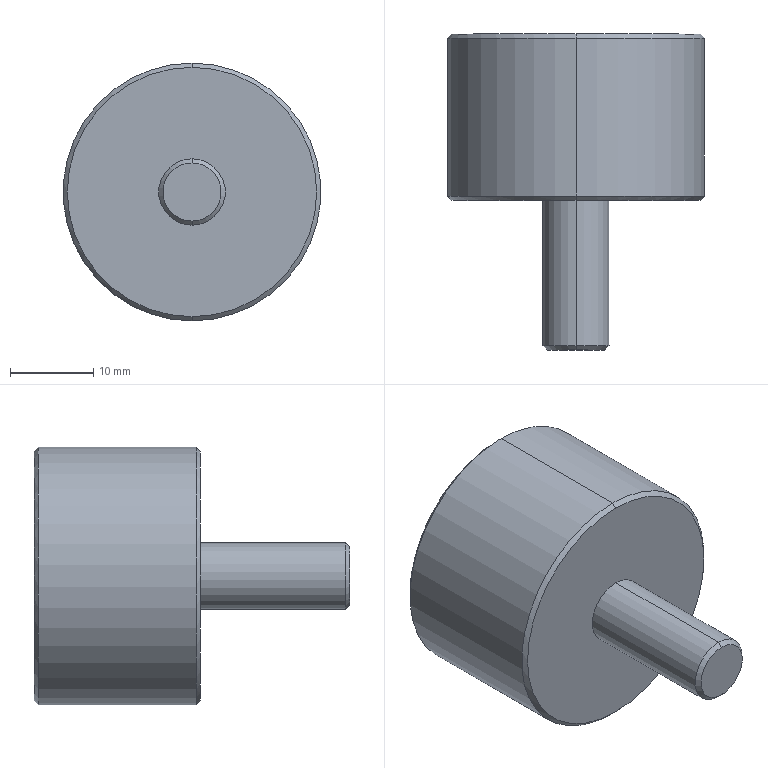Part | STEP file | OP10-123_seal rod | 1 solid | 23 faces | box 31 x 38 x 31 mm | volume 15633 mm3 | cylinder 10 | cone 8 | plane 5 | commonest cylinder face diameters 3.3 x2 6 x2 8 x2 11 x2 31 x2
STEP:
#1=CARTESIAN_POINT('',(0.,0.,0.));
#2=DIRECTION('',(0.,0.,1.));
#3=DIRECTION('',(1.,0.,0.));
#4=AXIS2_PLACEMENT_3D('',#1,#2,#3);
#5=CARTESIAN_POINT('',(0.,0.,-3.5));
#6=VERTEX_POINT('',#5);
#7=CARTESIAN_POINT('',(0.,0.,3.5));
#8=VERTEX_POINT('',#7);
#9=CARTESIAN_POINT('',(0.,0.,0.));
#10=DIRECTION('',(0.,-1.,0.));
#11=DIRECTION('',(0.,0.,1.));
#12=AXIS2_PLACEMENT_3D('',#9,#10,#11);
#13=CIRCLE('',#12,3.5);
#14=CARTESIAN_POINT('',(0.,0.5,0.));
#15=DIRECTION('',(0.,1.,0.));
#16=DIRECTION('',(0.,0.,1.));
#17=AXIS2_PLACEMENT_3D('',#14,#15,#16);
#18=CONICAL_SURFACE('',#17,4.,0.7854);
#19=CARTESIAN_POINT('',(6.283,-0.5));
#20=DIRECTION('',(-1.,0.));
#21=VECTOR('',#20,1.);
#22=LINE('',#19,#21);
#23=(GEOMETRIC_REPRESENTATION_CONTEXT(2)PARAMETRIC_REPRESENTATION_CONTEXT()REPRESENTATION_CONTEXT('',''));
#24=DEFINITIONAL_REPRESENTATION('',(#22),#23);
#25=PCURVE('',#18,#24);
#26=CARTESIAN_POINT('',(0.,0.,0.));
#27=DIRECTION('',(0.,1.,0.));
#28=DIRECTION('',(0.,0.,1.));
#29=AXIS2_PLACEMENT_3D('',#26,#27,#28);
#30=PLANE('',#29);
#31=CARTESIAN_POINT('',(3.5,0.));
#32=CARTESIAN_POINT('',(3.5,-6.062));
#33=CARTESIAN_POINT('',(-1.75,-3.031));
#34=CARTESIAN_POINT('',(-7.,0.));
#35=CARTESIAN_POINT('',(-1.75,3.031));
#36=CARTESIAN_POINT('',(3.5,6.062));
#37=CARTESIAN_POINT('',(3.5,0.));
#38=(BOUNDED_CURVE()B_SPLINE_CURVE(2,(#31,#32,#33,#34,#35,#36,#37),.UNSPECIFIED.,.T.,.F.)B_SPLINE_CURVE_WITH_KNOTS((1,2,2,2,2,1),(-2.094,0.,2.094,4.189,6.283,8.378),.UNSPECIFIED.)CURVE()GEOMETRIC_REPRESENTATION_ITEM()RATIONAL_B_SPLINE_CURVE((1.,0.5,1.,0.5,1.,0.5,1.))REPRESENTATION_ITEM(''));
#39=(GEOMETRIC_REPRESENTATION_CONTEXT(2)PARAMETRIC_REPRESENTATION_CONTEXT()REPRESENTATION_CONTEXT('',''));
#40=DEFINITIONAL_REPRESENTATION('',(#38),#39);
#41=PCURVE('',#30,#40);
#42=SURFACE_CURVE('',#13,(#25,#41),.PCURVE_S1.);
#43=EDGE_CURVE('',#6,#8,#42,.T.);
#44=ORIENTED_EDGE('',*,*,#43,.F.);
#45=CARTESIAN_POINT('',(0.,0.5,-4.));
#46=VERTEX_POINT('',#45);
#47=CARTESIAN_POINT('',(0.,0.5,-4.));
#48=DIRECTION('',(0.,0.7071,-0.7071));
#49=VECTOR('',#48,1.);
#50=LINE('',#47,#49);
#51=CARTESIAN_POINT('',(3.142,0.));
#52=DIRECTION('',(0.,1.));
#53=VECTOR('',#52,1.);
#54=LINE('',#51,#53);
#55=(GEOMETRIC_REPRESENTATION_CONTEXT(2)PARAMETRIC_REPRESENTATION_CONTEXT()REPRESENTATION_CONTEXT('',''));
#56=DEFINITIONAL_REPRESENTATION('',(#54),#55);
#57=PCURVE('',#18,#56);
#58=CARTESIAN_POINT('',(0.,0.5,0.));
#59=DIRECTION('',(0.,1.,0.));
#60=DIRECTION('',(0.,0.,1.));
#61=AXIS2_PLACEMENT_3D('',#58,#59,#60);
#62=CONICAL_SURFACE('',#61,4.,0.7854);
#63=CARTESIAN_POINT('',(3.142,0.));
#64=DIRECTION('',(0.,1.));
#65=VECTOR('',#64,1.);
#66=LINE('',#63,#65);
#67=(GEOMETRIC_REPRESENTATION_CONTEXT(2)PARAMETRIC_REPRESENTATION_CONTEXT()REPRESENTATION_CONTEXT('',''));
#68=DEFINITIONAL_REPRESENTATION('',(#66),#67);
#69=PCURVE('',#62,#68);
#70=SURFACE_CURVE('',#50,(#57,#69),.PCURVE_S1.);
#71=EDGE_CURVE('',#6,#46,#70,.T.);
#72=ORIENTED_EDGE('',*,*,#71,.T.);
#73=CARTESIAN_POINT('',(0.,0.5,4.));
#74=VERTEX_POINT('',#73);
#75=CARTESIAN_POINT('',(0.,0.5,0.));
#76=DIRECTION('',(0.,1.,0.));
#77=DIRECTION('',(0.,0.,1.));
#78=AXIS2_PLACEMENT_3D('',#75,#76,#77);
#79=CIRCLE('',#78,4.);
#80=CARTESIAN_POINT('',(0.,0.));
#81=DIRECTION('',(1.,0.));
#82=VECTOR('',#81,1.);
#83=LINE('',#80,#82);
#84=(GEOMETRIC_REPRESENTATION_CONTEXT(2)PARAMETRIC_REPRESENTATION_CONTEXT()REPRESENTATION_CONTEXT('',''));
#85=DEFINITIONAL_REPRESENTATION('',(#83),#84);
#86=PCURVE('',#18,#85);
#87=CARTESIAN_POINT('',(0.,18.,0.));
#88=DIRECTION('',(0.,-1.,0.));
#89=DIRECTION('',(0.,0.,-1.));
#90=AXIS2_PLACEMENT_3D('',#87,#88,#89);
#91=CYLINDRICAL_SURFACE('',#90,4.);
#92=CARTESIAN_POINT('',(3.142,17.5));
#93=DIRECTION('',(-1.,0.));
#94=VECTOR('',#93,1.);
#95=LINE('',#92,#94);
#96=(GEOMETRIC_REPRESENTATION_CONTEXT(2)PARAMETRIC_REPRESENTATION_CONTEXT()REPRESENTATION_CONTEXT('',''));
#97=DEFINITIONAL_REPRESENTATION('',(#95),#96);
#98=PCURVE('',#91,#97);
#99=SURFACE_CURVE('',#79,(#86,#98),.PCURVE_S1.);
#100=EDGE_CURVE('',#74,#46,#99,.T.);
#101=ORIENTED_EDGE('',*,*,#100,.F.);
#102=CARTESIAN_POINT('',(0.,0.5,4.));
#103=DIRECTION('',(0.,0.7071,0.7071));
#104=VECTOR('',#103,1.);
#105=LINE('',#102,#104);
#106=CARTESIAN_POINT('',(0.,0.));
#107=DIRECTION('',(0.,1.));
#108=VECTOR('',#107,1.);
#109=LINE('',#106,#108);
#110=(GEOMETRIC_REPRESENTATION_CONTEXT(2)PARAMETRIC_REPRESENTATION_CONTEXT()REPRESENTATION_CONTEXT('',''));
#111=DEFINITIONAL_REPRESENTATION('',(#109),#110);
#112=PCURVE('',#18,#111);
#113=CARTESIAN_POINT('',(6.283,0.));
#114=DIRECTION('',(0.,1.));
#115=VECTOR('',#114,1.);
#116=LINE('',#113,#115);
#117=(GEOMETRIC_REPRESENTATION_CONTEXT(2)PARAMETRIC_REPRESENTATION_CONTEXT()REPRESENTATION_CONTEXT('',''));
#118=DEFINITIONAL_REPRESENTATION('',(#116),#117);
#119=PCURVE('',#62,#118);
#120=SURFACE_CURVE('',#105,(#112,#119),.PCURVE_S1.);
#121=EDGE_CURVE('',#8,#74,#120,.T.);
#122=ORIENTED_EDGE('',*,*,#121,.F.);
#123=EDGE_LOOP('',(#44,#72,#101,#122));
#124=FACE_BOUND('',#123,.T.);
#125=ADVANCED_FACE('',(#124),#18,.T.);
#126=CARTESIAN_POINT('',(0.,38.,15.));
#127=VERTEX_POINT('',#126);
#128=CARTESIAN_POINT('',(0.,38.,-15.));
#129=VERTEX_POINT('',#128);
#130=CARTESIAN_POINT('',(0.,38.,0.));
#131=DIRECTION('',(0.,1.,0.));
#132=DIRECTION('',(0.,0.,1.));
#133=AXIS2_PLACEMENT_3D('',#130,#131,#132);
#134=CIRCLE('',#133,15.);
#135=CARTESIAN_POINT('',(0.,38.,0.));
#136=DIRECTION('',(0.,-1.,0.));
#137=DIRECTION('',(0.,0.,-1.));
#138=AXIS2_PLACEMENT_3D('',#135,#136,#137);
#139=CONICAL_SURFACE('',#138,15.,0.7854);
#140=CARTESIAN_POINT('',(3.142,0.));
#141=DIRECTION('',(-1.,0.));
#142=VECTOR('',#141,1.);
#143=LINE('',#140,#142);
#144=(GEOMETRIC_REPRESENTATION_CONTEXT(2)PARAMETRIC_REPRESENTATION_CONTEXT()REPRESENTATION_CONTEXT('',''));
#145=DEFINITIONAL_REPRESENTATION('',(#143),#144);
#146=PCURVE('',#139,#145);
#147=CARTESIAN_POINT('',(0.,38.,0.));
#148=DIRECTION('',(0.,1.,0.));
#149=DIRECTION('',(0.,0.,1.));
#150=AXIS2_PLACEMENT_3D('',#147,#148,#149);
#151=PLANE('',#150);
#152=CARTESIAN_POINT('',(0.,0.));
#153=DIRECTION('',(1.,0.));
#154=AXIS2_PLACEMENT_2D('',#152,#153);
#155=CIRCLE('',#154,15.);
#156=(GEOMETRIC_REPRESENTATION_CONTEXT(2)PARAMETRIC_REPRESENTATION_CONTEXT()REPRESENTATION_CONTEXT('',''));
#157=DEFINITIONAL_REPRESENTATION('',(#155),#156);
#158=PCURVE('',#151,#157);
#159=SURFACE_CURVE('',#134,(#146,#158),.PCURVE_S1.);
#160=EDGE_CURVE('',#127,#129,#159,.T.);
#161=ORIENTED_EDGE('',*,*,#160,.F.);
#162=CARTESIAN_POINT('',(0.,37.5,15.5));
#163=VERTEX_POINT('',#162);
#164=CARTESIAN_POINT('',(0.,38.,15.));
#165=DIRECTION('',(0.,-0.7071,0.7071));
#166=VECTOR('',#165,1.);
#167=LINE('',#164,#166);
#168=CARTESIAN_POINT('',(3.142,0.));
#169=DIRECTION('',(0.,1.));
#170=VECTOR('',#169,1.);
#171=LINE('',#168,#170);
#172=(GEOMETRIC_REPRESENTATION_CONTEXT(2)PARAMETRIC_REPRESENTATION_CONTEXT()REPRESENTATION_CONTEXT('',''));
#173=DEFINITIONAL_REPRESENTATION('',(#171),#172);
#174=PCURVE('',#139,#173);
#175=CARTESIAN_POINT('',(0.,38.,0.));
#176=DIRECTION('',(0.,-1.,0.));
#177=DIRECTION('',(0.,0.,-1.));
#178=AXIS2_PLACEMENT_3D('',#175,#176,#177);
#179=CONICAL_SURFACE('',#178,15.,0.7854);
#180=CARTESIAN_POINT('',(3.142,0.));
#181=DIRECTION('',(0.,1.));
#182=VECTOR('',#181,1.);
#183=LINE('',#180,#182);
#184=(GEOMETRIC_REPRESENTATION_CONTEXT(2)PARAMETRIC_REPRESENTATION_CONTEXT()REPRESENTATION_CONTEXT('',''));
#185=DEFINITIONAL_REPRESENTATION('',(#183),#184);
#186=PCURVE('',#179,#185);
#187=SURFACE_CURVE('',#167,(#174,#186),.PCURVE_S1.);
#188=EDGE_CURVE('',#127,#163,#187,.T.);
#189=ORIENTED_EDGE('',*,*,#188,.T.);
#190=CARTESIAN_POINT('',(0.,37.5,-15.5));
#191=VERTEX_POINT('',#190);
#192=CARTESIAN_POINT('',(0.,37.5,0.));
#193=DIRECTION('',(0.,-1.,0.));
#194=DIRECTION('',(0.,0.,1.));
#195=AXIS2_PLACEMENT_3D('',#192,#193,#194);
#196=CIRCLE('',#195,15.5);
#197=CARTESIAN_POINT('',(-3.142,0.5));
#198=DIRECTION('',(1.,0.));
#199=VECTOR('',#198,1.);
#200=LINE('',#197,#199);
#201=(GEOMETRIC_REPRESENTATION_CONTEXT(2)PARAMETRIC_REPRESENTATION_CONTEXT()REPRESENTATION_CONTEXT('',''));
#202=DEFINITIONAL_REPRESENTATION('',(#200),#201);
#203=PCURVE('',#139,#202);
#204=CARTESIAN_POINT('',(0.,38.,0.));
#205=DIRECTION('',(0.,-1.,0.));
#206=DIRECTION('',(0.,0.,-1.));
#207=AXIS2_PLACEMENT_3D('',#204,#205,#206);
#208=CYLINDRICAL_SURFACE('',#207,15.5);
#209=CARTESIAN_POINT('',(-3.142,0.5));
#210=DIRECTION('',(1.,0.));
#211=VECTOR('',#210,1.);
#212=LINE('',#209,#211);
#213=(GEOMETRIC_REPRESENTATION_CONTEXT(2)PARAMETRIC_REPRESENTATION_CONTEXT()REPRESENTATION_CONTEXT('',''));
#214=DEFINITIONAL_REPRESENTATION('',(#212),#213);
#215=PCURVE('',#208,#214);
#216=SURFACE_CURVE('',#196,(#203,#215),.PCURVE_S1.);
#217=EDGE_CURVE('',#191,#163,#216,.T.);
#218=ORIENTED_EDGE('',*,*,#217,.F.);
#219=CARTESIAN_POINT('',(0.,38.,-15.));
#220=DIRECTION('',(0.,-0.7071,-0.7071));
#221=VECTOR('',#220,1.);
#222=LINE('',#219,#221);
#223=CARTESIAN_POINT('',(0.,0.));
#224=DIRECTION('',(0.,1.));
#225=VECTOR('',#224,1.);
#226=LINE('',#223,#225);
#227=(GEOMETRIC_REPRESENTATION_CONTEXT(2)PARAMETRIC_REPRESENTATION_CONTEXT()REPRESENTATION_CONTEXT('',''));
#228=DEFINITIONAL_REPRESENTATION('',(#226),#227);
#229=PCURVE('',#139,#228);
#230=CARTESIAN_POINT('',(6.283,0.));
#231=DIRECTION('',(0.,1.));
#232=VECTOR('',#231,1.);
#233=LINE('',#230,#232);
#234=(GEOMETRIC_REPRESENTATION_CONTEXT(2)PARAMETRIC_REPRESENTATION_CONTEXT()REPRESENTATION_CONTEXT('',''));
#235=DEFINITIONAL_REPRESENTATION('',(#233),#234);
#236=PCURVE('',#179,#235);
#237=SURFACE_CURVE('',#222,(#229,#236),.PCURVE_S1.);
#238=EDGE_CURVE('',#129,#191,#237,.T.);
#239=ORIENTED_EDGE('',*,*,#238,.F.);
#240=EDGE_LOOP('',(#161,#189,#218,#239));
#241=FACE_BOUND('',#240,.T.);
#242=ADVANCED_FACE('',(#241),#139,.T.);
#243=CARTESIAN_POINT('',(0.,18.,-15.));
#244=VERTEX_POINT('',#243);
#245=CARTESIAN_POINT('',(0.,18.,15.));
#246=VERTEX_POINT('',#245);
#247=CARTESIAN_POINT('',(0.,18.,0.));
#248=DIRECTION('',(0.,-1.,0.));
#249=DIRECTION('',(0.,0.,1.));
#250=AXIS2_PLACEMENT_3D('',#247,#248,#249);
#251=CIRCLE('',#250,15.);
#252=CARTESIAN_POINT('',(0.,18.5,0.));
#253=DIRECTION('',(0.,1.,0.));
#254=DIRECTION('',(0.,0.,1.));
#255=AXIS2_PLACEMENT_3D('',#252,#253,#254);
#256=CONICAL_SURFACE('',#255,15.5,0.7854);
#257=CARTESIAN_POINT('',(6.283,-0.5));
#258=DIRECTION('',(-1.,0.));
#259=VECTOR('',#258,1.);
#260=LINE('',#257,#259);
#261=(GEOMETRIC_REPRESENTATION_CONTEXT(2)PARAMETRIC_REPRESENTATION_CONTEXT()REPRESENTATION_CONTEXT('',''));
#262=DEFINITIONAL_REPRESENTATION('',(#260),#261);
#263=PCURVE('',#256,#262);
#264=CARTESIAN_POINT('',(0.,18.,0.));
#265=DIRECTION('',(0.,1.,0.));
#266=DIRECTION('',(0.,0.,1.));
#267=AXIS2_PLACEMENT_3D('',#264,#265,#266);
#268=PLANE('',#267);
#269=CARTESIAN_POINT('',(15.,0.));
#270=CARTESIAN_POINT('',(15.,-25.981));
#271=CARTESIAN_POINT('',(-7.5,-12.99));
#272=CARTESIAN_POINT('',(-30.,0.));
#273=CARTESIAN_POINT('',(-7.5,12.99));
#274=CARTESIAN_POINT('',(15.,25.981));
#275=CARTESIAN_POINT('',(15.,0.));
#276=(BOUNDED_CURVE()B_SPLINE_CURVE(2,(#269,#270,#271,#272,#273,#274,#275),.UNSPECIFIED.,.T.,.F.)B_SPLINE_CURVE_WITH_KNOTS((1,2,2,2,2,1),(-2.094,0.,2.094,4.189,6.283,8.378),.UNSPECIFIED.)CURVE()GEOMETRIC_REPRESENTATION_ITEM()RATIONAL_B_SPLINE_CURVE((1.,0.5,1.,0.5,1.,0.5,1.))REPRESENTATION_ITEM(''));
#277=(GEOMETRIC_REPRESENTATION_CONTEXT(2)PARAMETRIC_REPRESENTATION_CONTEXT()REPRESENTATION_CONTEXT('',''));
#278=DEFINITIONAL_REPRESENTATION('',(#276),#277);
#279=PCURVE('',#268,#278);
#280=SURFACE_CURVE('',#251,(#263,#279),.PCURVE_S1.);
#281=EDGE_CURVE('',#244,#246,#280,.T.);
#282=ORIENTED_EDGE('',*,*,#281,.F.);
#283=CARTESIAN_POINT('',(0.,18.5,-15.5));
#284=VERTEX_POINT('',#283);
#285=CARTESIAN_POINT('',(0.,18.5,-15.5));
#286=DIRECTION('',(0.,0.7071,-0.7071));
#287=VECTOR('',#286,1.);
#288=LINE('',#285,#287);
#289=CARTESIAN_POINT('',(3.142,0.));
#290=DIRECTION('',(0.,1.));
#291=VECTOR('',#290,1.);
#292=LINE('',#289,#291);
#293=(GEOMETRIC_REPRESENTATION_CONTEXT(2)PARAMETRIC_REPRESENTATION_CONTEXT()REPRESENTATION_CONTEXT('',''));
#294=DEFINITIONAL_REPRESENTATION('',(#292),#293);
#295=PCURVE('',#256,#294);
#296=CARTESIAN_POINT('',(0.,18.5,0.));
#297=DIRECTION('',(0.,1.,0.));
#298=DIRECTION('',(0.,0.,1.));
#299=AXIS2_PLACEMENT_3D('',#296,#297,#298);
#300=CONICAL_SURFACE('',#299,15.5,0.7854);
#301=CARTESIAN_POINT('',(3.142,0.));
#302=DIRECTION('',(0.,1.));
#303=VECTOR('',#302,1.);
#304=LINE('',#301,#303);
#305=(GEOMETRIC_REPRESENTATION_CONTEXT(2)PARAMETRIC_REPRESENTATION_CONTEXT()REPRESENTATION_CONTEXT('',''));
#306=DEFINITIONAL_REPRESENTATION('',(#304),#305);
#307=PCURVE('',#300,#306);
#308=SURFACE_CURVE('',#288,(#295,#307),.PCURVE_S1.);
#309=EDGE_CURVE('',#244,#284,#308,.T.);
#310=ORIENTED_EDGE('',*,*,#309,.T.);
#311=CARTESIAN_POINT('',(0.,18.5,15.5));
#312=VERTEX_POINT('',#311);
#313=CARTESIAN_POINT('',(0.,18.5,0.));
#314=DIRECTION('',(0.,1.,0.));
#315=DIRECTION('',(0.,0.,1.));
#316=AXIS2_PLACEMENT_3D('',#313,#314,#315);
#317=CIRCLE('',#316,15.5);
#318=CARTESIAN_POINT('',(0.,0.));
#319=DIRECTION('',(1.,0.));
#320=VECTOR('',#319,1.);
#321=LINE('',#318,#320);
#322=(GEOMETRIC_REPRESENTATION_CONTEXT(2)PARAMETRIC_REPRESENTATION_CONTEXT()REPRESENTATION_CONTEXT('',''));
#323=DEFINITIONAL_REPRESENTATION('',(#321),#322);
#324=PCURVE('',#256,#323);
#325=CARTESIAN_POINT('',(3.142,19.5));
#326=DIRECTION('',(-1.,0.));
#327=VECTOR('',#326,1.);
#328=LINE('',#325,#327);
#329=(GEOMETRIC_REPRESENTATION_CONTEXT(2)PARAMETRIC_REPRESENTATION_CONTEXT()REPRESENTATION_CONTEXT('',''));
#330=DEFINITIONAL_REPRESENTATION('',(#328),#329);
#331=PCURVE('',#208,#330);
#332=SURFACE_CURVE('',#317,(#324,#331),.PCURVE_S1.);
#333=EDGE_CURVE('',#312,#284,#332,.T.);
#334=ORIENTED_EDGE('',*,*,#333,.F.);
#335=CARTESIAN_POINT('',(0.,18.5,15.5));
#336=DIRECTION('',(0.,0.7071,0.7071));
#337=VECTOR('',#336,1.);
#338=LINE('',#335,#337);
#339=CARTESIAN_POINT('',(0.,0.));
#340=DIRECTION('',(0.,1.));
#341=VECTOR('',#340,1.);
#342=LINE('',#339,#341);
#343=(GEOMETRIC_REPRESENTATION_CONTEXT(2)PARAMETRIC_REPRESENTATION_CONTEXT()REPRESENTATION_CONTEXT('',''));
#344=DEFINITIONAL_REPRESENTATION('',(#342),#343);
#345=PCURVE('',#256,#344);
#346=CARTESIAN_POINT('',(6.283,0.));
#347=DIRECTION('',(0.,1.));
#348=VECTOR('',#347,1.);
#349=LINE('',#346,#348);
#350=(GEOMETRIC_REPRESENTATION_CONTEXT(2)PARAMETRIC_REPRESENTATION_CONTEXT()REPRESENTATION_CONTEXT('',''));
#351=DEFINITIONAL_REPRESENTATION('',(#349),#350);
#352=PCURVE('',#300,#351);
#353=SURFACE_CURVE('',#338,(#345,#352),.PCURVE_S1.);
#354=EDGE_CURVE('',#246,#312,#353,.T.);
#355=ORIENTED_EDGE('',*,*,#354,.F.);
#356=EDGE_LOOP('',(#282,#310,#334,#355));
#357=FACE_BOUND('',#356,.T.);
#358=ADVANCED_FACE('',(#357),#256,.T.);
#359=CARTESIAN_POINT('',(0.,21.,1.65));
#360=VERTEX_POINT('',#359);
#361=CARTESIAN_POINT('',(0.,33.,1.65));
#362=VERTEX_POINT('',#361);
#363=CARTESIAN_POINT('',(0.,33.,1.65));
#364=DIRECTION('',(0.,1.,0.));
#365=VECTOR('',#364,1.);
#366=LINE('',#363,#365);
#367=CARTESIAN_POINT('',(0.,33.,0.));
#368=DIRECTION('',(0.,1.,0.));
#369=DIRECTION('',(0.,0.,1.));
#370=AXIS2_PLACEMENT_3D('',#367,#368,#369);
#371=CYLINDRICAL_SURFACE('',#370,1.65);
#372=CARTESIAN_POINT('',(6.283,0.));
#373=DIRECTION('',(0.,1.));
#374=VECTOR('',#373,1.);
#375=LINE('',#372,#374);
#376=(GEOMETRIC_REPRESENTATION_CONTEXT(2)PARAMETRIC_REPRESENTATION_CONTEXT()REPRESENTATION_CONTEXT('',''));
#377=DEFINITIONAL_REPRESENTATION('',(#375),#376);
#378=PCURVE('',#371,#377);
#379=CARTESIAN_POINT('',(0.,33.,0.));
#380=DIRECTION('',(0.,1.,0.));
#381=DIRECTION('',(0.,0.,1.));
#382=AXIS2_PLACEMENT_3D('',#379,#380,#381);
#383=CYLINDRICAL_SURFACE('',#382,1.65);
#384=CARTESIAN_POINT('',(0.,0.));
#385=DIRECTION('',(0.,1.));
#386=VECTOR('',#385,1.);
#387=LINE('',#384,#386);
#388=(GEOMETRIC_REPRESENTATION_CONTEXT(2)PARAMETRIC_REPRESENTATION_CONTEXT()REPRESENTATION_CONTEXT('',''));
#389=DEFINITIONAL_REPRESENTATION('',(#387),#388);
#390=PCURVE('',#383,#389);
#391=SURFACE_CURVE('',#366,(#378,#390),.PCURVE_S1.);
#392=EDGE_CURVE('',#360,#362,#391,.T.);
#393=ORIENTED_EDGE('',*,*,#392,.T.);
#394=CARTESIAN_POINT('',(0.,33.,-1.65));
#395=VERTEX_POINT('',#394);
#396=CARTESIAN_POINT('',(0.,33.,0.));
#397=DIRECTION('',(0.,1.,0.));
#398=DIRECTION('',(0.,0.,1.));
#399=AXIS2_PLACEMENT_3D('',#396,#397,#398);
#400=CIRCLE('',#399,1.65);
#401=CARTESIAN_POINT('',(0.,0.));
#402=DIRECTION('',(1.,0.));
#403=VECTOR('',#402,1.);
#404=LINE('',#401,#403);
#405=(GEOMETRIC_REPRESENTATION_CONTEXT(2)PARAMETRIC_REPRESENTATION_CONTEXT()REPRESENTATION_CONTEXT('',''));
#406=DEFINITIONAL_REPRESENTATION('',(#404),#405);
#407=PCURVE('',#371,#406);
#408=CARTESIAN_POINT('',(0.,33.,0.));
#409=DIRECTION('',(0.,1.,0.));
#410=DIRECTION('',(0.,0.,1.));
#411=AXIS2_PLACEMENT_3D('',#408,#409,#410);
#412=PLANE('',#411);
#413=CARTESIAN_POINT('',(0.,0.));
#414=DIRECTION('',(1.,0.));
#415=AXIS2_PLACEMENT_2D('',#413,#414);
#416=CIRCLE('',#415,1.65);
#417=(GEOMETRIC_REPRESENTATION_CONTEXT(2)PARAMETRIC_REPRESENTATION_CONTEXT()REPRESENTATION_CONTEXT('',''));
#418=DEFINITIONAL_REPRESENTATION('',(#416),#417);
#419=PCURVE('',#412,#418);
#420=SURFACE_CURVE('',#400,(#407,#419),.PCURVE_S1.);
#421=EDGE_CURVE('',#395,#362,#420,.T.);
#422=ORIENTED_EDGE('',*,*,#421,.F.);
#423=CARTESIAN_POINT('',(0.,21.,-1.65));
#424=VERTEX_POINT('',#423);
#425=CARTESIAN_POINT('',(0.,33.,-1.65));
#426=DIRECTION('',(0.,1.,0.));
#427=VECTOR('',#426,1.);
#428=LINE('',#425,#427);
#429=CARTESIAN_POINT('',(3.142,0.));
#430=DIRECTION('',(0.,1.));
#431=VECTOR('',#430,1.);
#432=LINE('',#429,#431);
#433=(GEOMETRIC_REPRESENTATION_CONTEXT(2)PARAMETRIC_REPRESENTATION_CONTEXT()REPRESENTATION_CONTEXT('',''));
#434=DEFINITIONAL_REPRESENTATION('',(#432),#433);
#435=PCURVE('',#371,#434);
#436=CARTESIAN_POINT('',(3.142,0.));
#437=DIRECTION('',(0.,1.));
#438=VECTOR('',#437,1.);
#439=LINE('',#436,#438);
#440=(GEOMETRIC_REPRESENTATION_CONTEXT(2)PARAMETRIC_REPRESENTATION_CONTEXT()REPRESENTATION_CONTEXT('',''));
#441=DEFINITIONAL_REPRESENTATION('',(#439),#440);
#442=PCURVE('',#383,#441);
#443=SURFACE_CURVE('',#428,(#435,#442),.PCURVE_S1.);
#444=EDGE_CURVE('',#424,#395,#443,.T.);
#445=ORIENTED_EDGE('',*,*,#444,.F.);
#446=CARTESIAN_POINT('',(0.,21.,0.));
#447=DIRECTION('',(0.,1.,0.));
#448=DIRECTION('',(0.,0.,1.));
#449=AXIS2_PLACEMENT_3D('',#446,#447,#448);
#450=CIRCLE('',#449,1.65);
#451=CARTESIAN_POINT('',(0.,-12.));
#452=DIRECTION('',(1.,0.));
#453=VECTOR('',#452,1.);
#454=LINE('',#451,#453);
#455=(GEOMETRIC_REPRESENTATION_CONTEXT(2)PARAMETRIC_REPRESENTATION_CONTEXT()REPRESENTATION_CONTEXT('',''));
#456=DEFINITIONAL_REPRESENTATION('',(#454),#455);
#457=PCURVE('',#371,#456);
#458=CARTESIAN_POINT('',(0.,21.,0.));
#459=DIRECTION('',(0.,1.,0.));
#460=DIRECTION('',(0.,0.,1.));
#461=AXIS2_PLACEMENT_3D('',#458,#459,#460);
#462=CONICAL_SURFACE('',#461,1.65,1.03);
#463=CARTESIAN_POINT('',(0.,0.));
#464=DIRECTION('',(1.,0.));
#465=VECTOR('',#464,1.);
#466=LINE('',#463,#465);
#467=(GEOMETRIC_REPRESENTATION_CONTEXT(2)PARAMETRIC_REPRESENTATION_CONTEXT()REPRESENTATION_CONTEXT('',''));
#468=DEFINITIONAL_REPRESENTATION('',(#466),#467);
#469=PCURVE('',#462,#468);
#470=SURFACE_CURVE('',#450,(#457,#469),.PCURVE_S1.);
#471=EDGE_CURVE('',#424,#360,#470,.T.);
#472=ORIENTED_EDGE('',*,*,#471,.T.);
#473=EDGE_LOOP('',(#393,#422,#445,#472));
#474=FACE_BOUND('',#473,.F.);
#475=ADVANCED_FACE('',(#474),#371,.F.);
#476=ORIENTED_EDGE('',*,*,#471,.F.);
#477=CARTESIAN_POINT('',(0.,20.009,0.));
#478=VERTEX_POINT('',#477);
#479=CARTESIAN_POINT('',(0.,21.,-1.65));
#480=DIRECTION('',(0.,0.515,-0.8572));
#481=VECTOR('',#480,1.);
#482=LINE('',#479,#481);
#483=CARTESIAN_POINT('',(3.142,0.));
#484=DIRECTION('',(0.,1.));
#485=VECTOR('',#484,1.);
#486=LINE('',#483,#485);
#487=(GEOMETRIC_REPRESENTATION_CONTEXT(2)PARAMETRIC_REPRESENTATION_CONTEXT()REPRESENTATION_CONTEXT('',''));
#488=DEFINITIONAL_REPRESENTATION('',(#486),#487);
#489=PCURVE('',#462,#488);
#490=CARTESIAN_POINT('',(0.,21.,0.));
#491=DIRECTION('',(0.,1.,0.));
#492=DIRECTION('',(0.,0.,1.));
#493=AXIS2_PLACEMENT_3D('',#490,#491,#492);
#494=CONICAL_SURFACE('',#493,1.65,1.03);
#495=CARTESIAN_POINT('',(3.142,0.));
#496=DIRECTION('',(0.,1.));
#497=VECTOR('',#496,1.);
#498=LINE('',#495,#497);
#499=(GEOMETRIC_REPRESENTATION_CONTEXT(2)PARAMETRIC_REPRESENTATION_CONTEXT()REPRESENTATION_CONTEXT('',''));
#500=DEFINITIONAL_REPRESENTATION('',(#498),#499);
#501=PCURVE('',#494,#500);
#502=SURFACE_CURVE('',#482,(#489,#501),.PCURVE_S1.);
#503=EDGE_CURVE('',#478,#424,#502,.T.);
#504=ORIENTED_EDGE('',*,*,#503,.F.);
#505=CARTESIAN_POINT('',(0.,21.,1.65));
#506=DIRECTION('',(0.,0.515,0.8572));
#507=VECTOR('',#506,1.);
#508=LINE('',#505,#507);
#509=CARTESIAN_POINT('',(6.283,0.));
#510=DIRECTION('',(0.,1.));
#511=VECTOR('',#510,1.);
#512=LINE('',#509,#511);
#513=(GEOMETRIC_REPRESENTATION_CONTEXT(2)PARAMETRIC_REPRESENTATION_CONTEXT()REPRESENTATION_CONTEXT('',''));
#514=DEFINITIONAL_REPRESENTATION('',(#512),#513);
#515=PCURVE('',#462,#514);
#516=CARTESIAN_POINT('',(0.,0.));
#517=DIRECTION('',(0.,1.));
#518=VECTOR('',#517,1.);
#519=LINE('',#516,#518);
#520=(GEOMETRIC_REPRESENTATION_CONTEXT(2)PARAMETRIC_REPRESENTATION_CONTEXT()REPRESENTATION_CONTEXT('',''));
#521=DEFINITIONAL_REPRESENTATION('',(#519),#520);
#522=PCURVE('',#494,#521);
#523=SURFACE_CURVE('',#508,(#515,#522),.PCURVE_S1.);
#524=EDGE_CURVE('',#478,#360,#523,.T.);
#525=ORIENTED_EDGE('',*,*,#524,.T.);
#526=EDGE_LOOP('',(#476,#504,#525));
#527=FACE_BOUND('',#526,.F.);
#528=ADVANCED_FACE('',(#527),#462,.F.);
#529=CARTESIAN_POINT('',(0.,33.,3.));
#530=VERTEX_POINT('',#529);
#531=CARTESIAN_POINT('',(0.,36.6,3.));
#532=VERTEX_POINT('',#531);
#533=CARTESIAN_POINT('',(0.,33.,3.));
#534=DIRECTION('',(0.,1.,0.));
#535=VECTOR('',#534,1.);
#536=LINE('',#533,#535);
#537=CARTESIAN_POINT('',(0.,33.,0.));
#538=DIRECTION('',(0.,1.,0.));
#539=DIRECTION('',(0.,0.,1.));
#540=AXIS2_PLACEMENT_3D('',#537,#538,#539);
#541=CYLINDRICAL_SURFACE('',#540,3.);
#542=CARTESIAN_POINT('',(6.283,0.));
#543=DIRECTION('',(0.,1.));
#544=VECTOR('',#543,1.);
#545=LINE('',#542,#544);
#546=(GEOMETRIC_REPRESENTATION_CONTEXT(2)PARAMETRIC_REPRESENTATION_CONTEXT()REPRESENTATION_CONTEXT('',''));
#547=DEFINITIONAL_REPRESENTATION('',(#545),#546);
#548=PCURVE('',#541,#547);
#549=CARTESIAN_POINT('',(0.,33.,0.));
#550=DIRECTION('',(0.,1.,0.));
#551=DIRECTION('',(0.,0.,1.));
#552=AXIS2_PLACEMENT_3D('',#549,#550,#551);
#553=CYLINDRICAL_SURFACE('',#552,3.);
#554=CARTESIAN_POINT('',(0.,0.));
#555=DIRECTION('',(0.,1.));
#556=VECTOR('',#555,1.);
#557=LINE('',#554,#556);
#558=(GEOMETRIC_REPRESENTATION_CONTEXT(2)PARAMETRIC_REPRESENTATION_CONTEXT()REPRESENTATION_CONTEXT('',''));
#559=DEFINITIONAL_REPRESENTATION('',(#557),#558);
#560=PCURVE('',#553,#559);
#561=SURFACE_CURVE('',#536,(#548,#560),.PCURVE_S1.);
#562=EDGE_CURVE('',#530,#532,#561,.T.);
#563=ORIENTED_EDGE('',*,*,#562,.T.);
#564=CARTESIAN_POINT('',(0.,36.6,-3.));
#565=VERTEX_POINT('',#564);
#566=CARTESIAN_POINT('',(0.,36.6,0.));
#567=DIRECTION('',(0.,1.,0.));
#568=DIRECTION('',(0.,0.,1.));
#569=AXIS2_PLACEMENT_3D('',#566,#567,#568);
#570=CIRCLE('',#569,3.);
#571=CARTESIAN_POINT('',(0.,3.6));
#572=DIRECTION('',(1.,0.));
#573=VECTOR('',#572,1.);
#574=LINE('',#571,#573);
#575=(GEOMETRIC_REPRESENTATION_CONTEXT(2)PARAMETRIC_REPRESENTATION_CONTEXT()REPRESENTATION_CONTEXT('',''));
#576=DEFINITIONAL_REPRESENTATION('',(#574),#575);
#577=PCURVE('',#541,#576);
#578=CARTESIAN_POINT('',(0.,36.6,0.));
#579=DIRECTION('',(0.,1.,0.));
#580=DIRECTION('',(0.,0.,1.));
#581=AXIS2_PLACEMENT_3D('',#578,#579,#580);
#582=PLANE('',#581);
#583=CARTESIAN_POINT('',(0.,0.));
#584=DIRECTION('',(1.,0.));
#585=AXIS2_PLACEMENT_2D('',#583,#584);
#586=CIRCLE('',#585,3.);
#587=(GEOMETRIC_REPRESENTATION_CONTEXT(2)PARAMETRIC_REPRESENTATION_CONTEXT()REPRESENTATION_CONTEXT('',''));
#588=DEFINITIONAL_REPRESENTATION('',(#586),#587);
#589=PCURVE('',#582,#588);
#590=SURFACE_CURVE('',#570,(#577,#589),.PCURVE_S1.);
#591=EDGE_CURVE('',#565,#532,#590,.T.);
#592=ORIENTED_EDGE('',*,*,#591,.F.);
#593=CARTESIAN_POINT('',(0.,33.,-3.));
#594=VERTEX_POINT('',#593);
#595=CARTESIAN_POINT('',(0.,33.,-3.));
#596=DIRECTION('',(0.,1.,0.));
#597=VECTOR('',#596,1.);
#598=LINE('',#595,#597);
#599=CARTESIAN_POINT('',(3.142,0.));
#600=DIRECTION('',(0.,1.));
#601=VECTOR('',#600,1.);
#602=LINE('',#599,#601);
#603=(GEOMETRIC_REPRESENTATION_CONTEXT(2)PARAMETRIC_REPRESENTATION_CONTEXT()REPRESENTATION_CONTEXT('',''));
#604=DEFINITIONAL_REPRESENTATION('',(#602),#603);
#605=PCURVE('',#541,#604);
#606=CARTESIAN_POINT('',(3.142,0.));
#607=DIRECTION('',(0.,1.));
#608=VECTOR('',#607,1.);
#609=LINE('',#606,#608);
#610=(GEOMETRIC_REPRESENTATION_CONTEXT(2)PARAMETRIC_REPRESENTATION_CONTEXT()REPRESENTATION_CONTEXT('',''));
#611=DEFINITIONAL_REPRESENTATION('',(#609),#610);
#612=PCURVE('',#553,#611);
#613=SURFACE_CURVE('',#598,(#605,#612),.PCURVE_S1.);
#614=EDGE_CURVE('',#594,#565,#613,.T.);
#615=ORIENTED_EDGE('',*,*,#614,.F.);
#616=CARTESIAN_POINT('',(0.,33.,0.));
#617=DIRECTION('',(0.,1.,0.));
#618=DIRECTION('',(0.,0.,1.));
#619=AXIS2_PLACEMENT_3D('',#616,#617,#618);
#620=CIRCLE('',#619,3.);
#621=CARTESIAN_POINT('',(0.,0.));
#622=DIRECTION('',(1.,0.));
#623=VECTOR('',#622,1.);
#624=LINE('',#621,#623);
#625=(GEOMETRIC_REPRESENTATION_CONTEXT(2)PARAMETRIC_REPRESENTATION_CONTEXT()REPRESENTATION_CONTEXT('',''));
#626=DEFINITIONAL_REPRESENTATION('',(#624),#625);
#627=PCURVE('',#541,#626);
#628=CARTESIAN_POINT('',(0.,0.));
#629=DIRECTION('',(1.,0.));
#630=AXIS2_PLACEMENT_2D('',#628,#629);
#631=CIRCLE('',#630,3.);
#632=(GEOMETRIC_REPRESENTATION_CONTEXT(2)PARAMETRIC_REPRESENTATION_CONTEXT()REPRESENTATION_CONTEXT('',''));
#633=DEFINITIONAL_REPRESENTATION('',(#631),#632);
#634=PCURVE('',#412,#633);
#635=SURFACE_CURVE('',#620,(#627,#634),.PCURVE_S1.);
#636=EDGE_CURVE('',#594,#530,#635,.T.);
#637=ORIENTED_EDGE('',*,*,#636,.T.);
#638=EDGE_LOOP('',(#563,#592,#615,#637));
#639=FACE_BOUND('',#638,.F.);
#640=ADVANCED_FACE('',(#639),#541,.F.);
#641=CARTESIAN_POINT('',(0.,36.6,5.5));
#642=VERTEX_POINT('',#641);
#643=CARTESIAN_POINT('',(0.,38.,5.5));
#644=VERTEX_POINT('',#643);
#645=CARTESIAN_POINT('',(0.,36.6,5.5));
#646=DIRECTION('',(0.,1.,0.));
#647=VECTOR('',#646,1.);
#648=LINE('',#645,#647);
#649=CARTESIAN_POINT('',(0.,36.6,0.));
#650=DIRECTION('',(0.,1.,0.));
#651=DIRECTION('',(0.,0.,1.));
#652=AXIS2_PLACEMENT_3D('',#649,#650,#651);
#653=CYLINDRICAL_SURFACE('',#652,5.5);
#654=CARTESIAN_POINT('',(6.283,0.));
#655=DIRECTION('',(0.,1.));
#656=VECTOR('',#655,1.);
#657=LINE('',#654,#656);
#658=(GEOMETRIC_REPRESENTATION_CONTEXT(2)PARAMETRIC_REPRESENTATION_CONTEXT()REPRESENTATION_CONTEXT('',''));
#659=DEFINITIONAL_REPRESENTATION('',(#657),#658);
#660=PCURVE('',#653,#659);
#661=CARTESIAN_POINT('',(0.,36.6,0.));
#662=DIRECTION('',(0.,1.,0.));
#663=DIRECTION('',(0.,0.,1.));
#664=AXIS2_PLACEMENT_3D('',#661,#662,#663);
#665=CYLINDRICAL_SURFACE('',#664,5.5);
#666=CARTESIAN_POINT('',(0.,0.));
#667=DIRECTION('',(0.,1.));
#668=VECTOR('',#667,1.);
#669=LINE('',#666,#668);
#670=(GEOMETRIC_REPRESENTATION_CONTEXT(2)PARAMETRIC_REPRESENTATION_CONTEXT()REPRESENTATION_CONTEXT('',''));
#671=DEFINITIONAL_REPRESENTATION('',(#669),#670);
#672=PCURVE('',#665,#671);
#673=SURFACE_CURVE('',#648,(#660,#672),.PCURVE_S1.);
#674=EDGE_CURVE('',#642,#644,#673,.T.);
#675=ORIENTED_EDGE('',*,*,#674,.T.);
#676=CARTESIAN_POINT('',(0.,38.,-5.5));
#677=VERTEX_POINT('',#676);
#678=CARTESIAN_POINT('',(0.,38.,0.));
#679=DIRECTION('',(0.,1.,0.));
#680=DIRECTION('',(0.,0.,1.));
#681=AXIS2_PLACEMENT_3D('',#678,#679,#680);
#682=CIRCLE('',#681,5.5);
#683=CARTESIAN_POINT('',(0.,1.4));
#684=DIRECTION('',(1.,0.));
#685=VECTOR('',#684,1.);
#686=LINE('',#683,#685);
#687=(GEOMETRIC_REPRESENTATION_CONTEXT(2)PARAMETRIC_REPRESENTATION_CONTEXT()REPRESENTATION_CONTEXT('',''));
#688=DEFINITIONAL_REPRESENTATION('',(#686),#687);
#689=PCURVE('',#653,#688);
#690=CARTESIAN_POINT('',(0.,0.));
#691=DIRECTION('',(1.,0.));
#692=AXIS2_PLACEMENT_2D('',#690,#691);
#693=CIRCLE('',#692,5.5);
#694=(GEOMETRIC_REPRESENTATION_CONTEXT(2)PARAMETRIC_REPRESENTATION_CONTEXT()REPRESENTATION_CONTEXT('',''));
#695=DEFINITIONAL_REPRESENTATION('',(#693),#694);
#696=PCURVE('',#151,#695);
#697=SURFACE_CURVE('',#682,(#689,#696),.PCURVE_S1.);
#698=EDGE_CURVE('',#677,#644,#697,.T.);
#699=ORIENTED_EDGE('',*,*,#698,.F.);
#700=CARTESIAN_POINT('',(0.,36.6,-5.5));
#701=VERTEX_POINT('',#700);
#702=CARTESIAN_POINT('',(0.,36.6,-5.5));
#703=DIRECTION('',(0.,1.,0.));
#704=VECTOR('',#703,1.);
#705=LINE('',#702,#704);
#706=CARTESIAN_POINT('',(3.142,0.));
#707=DIRECTION('',(0.,1.));
#708=VECTOR('',#707,1.);
#709=LINE('',#706,#708);
#710=(GEOMETRIC_REPRESENTATION_CONTEXT(2)PARAMETRIC_REPRESENTATION_CONTEXT()REPRESENTATION_CONTEXT('',''));
#711=DEFINITIONAL_REPRESENTATION('',(#709),#710);
#712=PCURVE('',#653,#711);
#713=CARTESIAN_POINT('',(3.142,0.));
#714=DIRECTION('',(0.,1.));
#715=VECTOR('',#714,1.);
#716=LINE('',#713,#715);
#717=(GEOMETRIC_REPRESENTATION_CONTEXT(2)PARAMETRIC_REPRESENTATION_CONTEXT()REPRESENTATION_CONTEXT('',''));
#718=DEFINITIONAL_REPRESENTATION('',(#716),#717);
#719=PCURVE('',#665,#718);
#720=SURFACE_CURVE('',#705,(#712,#719),.PCURVE_S1.);
#721=EDGE_CURVE('',#701,#677,#720,.T.);
#722=ORIENTED_EDGE('',*,*,#721,.F.);
#723=CARTESIAN_POINT('',(0.,36.6,0.));
#724=DIRECTION('',(0.,1.,0.));
#725=DIRECTION('',(0.,0.,1.));
#726=AXIS2_PLACEMENT_3D('',#723,#724,#725);
#727=CIRCLE('',#726,5.5);
#728=CARTESIAN_POINT('',(0.,0.));
#729=DIRECTION('',(1.,0.));
#730=VECTOR('',#729,1.);
#731=LINE('',#728,#730);
#732=(GEOMETRIC_REPRESENTATION_CONTEXT(2)PARAMETRIC_REPRESENTATION_CONTEXT()REPRESENTATION_CONTEXT('',''));
#733=DEFINITIONAL_REPRESENTATION('',(#731),#732);
#734=PCURVE('',#653,#733);
#735=CARTESIAN_POINT('',(0.,0.));
#736=DIRECTION('',(1.,0.));
#737=AXIS2_PLACEMENT_2D('',#735,#736);
#738=CIRCLE('',#737,5.5);
#739=(GEOMETRIC_REPRESENTATION_CONTEXT(2)PARAMETRIC_REPRESENTATION_CONTEXT()REPRESENTATION_CONTEXT('',''));
#740=DEFINITIONAL_REPRESENTATION('',(#738),#739);
#741=PCURVE('',#582,#740);
#742=SURFACE_CURVE('',#727,(#734,#741),.PCURVE_S1.);
#743=EDGE_CURVE('',#701,#642,#742,.T.);
#744=ORIENTED_EDGE('',*,*,#743,.T.);
#745=EDGE_LOOP('',(#675,#699,#722,#744));
#746=FACE_BOUND('',#745,.F.);
#747=ADVANCED_FACE('',(#746),#653,.F.);
#748=ORIENTED_EDGE('',*,*,#217,.T.);
#749=CARTESIAN_POINT('',(0.,38.,15.5));
#750=DIRECTION('',(0.,-1.,0.));
#751=VECTOR('',#750,1.);
#752=LINE('',#749,#751);
#753=CARTESIAN_POINT('',(3.142,0.));
#754=DIRECTION('',(0.,1.));
#755=VECTOR('',#754,1.);
#756=LINE('',#753,#755);
#757=(GEOMETRIC_REPRESENTATION_CONTEXT(2)PARAMETRIC_REPRESENTATION_CONTEXT()REPRESENTATION_CONTEXT('',''));
#758=DEFINITIONAL_REPRESENTATION('',(#756),#757);
#759=PCURVE('',#208,#758);
#760=CARTESIAN_POINT('',(0.,38.,0.));
#761=DIRECTION('',(0.,-1.,0.));
#762=DIRECTION('',(0.,0.,-1.));
#763=AXIS2_PLACEMENT_3D('',#760,#761,#762);
#764=CYLINDRICAL_SURFACE('',#763,15.5);
#765=CARTESIAN_POINT('',(3.142,0.));
#766=DIRECTION('',(0.,1.));
#767=VECTOR('',#766,1.);
#768=LINE('',#765,#767);
#769=(GEOMETRIC_REPRESENTATION_CONTEXT(2)PARAMETRIC_REPRESENTATION_CONTEXT()REPRESENTATION_CONTEXT('',''));
#770=DEFINITIONAL_REPRESENTATION('',(#768),#769);
#771=PCURVE('',#764,#770);
#772=SURFACE_CURVE('',#752,(#759,#771),.PCURVE_S1.);
#773=EDGE_CURVE('',#163,#312,#772,.T.);
#774=ORIENTED_EDGE('',*,*,#773,.T.);
#775=ORIENTED_EDGE('',*,*,#333,.T.);
#776=CARTESIAN_POINT('',(0.,38.,-15.5));
#777=DIRECTION('',(0.,-1.,0.));
#778=VECTOR('',#777,1.);
#779=LINE('',#776,#778);
#780=CARTESIAN_POINT('',(0.,0.));
#781=DIRECTION('',(0.,1.));
#782=VECTOR('',#781,1.);
#783=LINE('',#780,#782);
#784=(GEOMETRIC_REPRESENTATION_CONTEXT(2)PARAMETRIC_REPRESENTATION_CONTEXT()REPRESENTATION_CONTEXT('',''));
#785=DEFINITIONAL_REPRESENTATION('',(#783),#784);
#786=PCURVE('',#208,#785);
#787=CARTESIAN_POINT('',(6.283,0.));
#788=DIRECTION('',(0.,1.));
#789=VECTOR('',#788,1.);
#790=LINE('',#787,#789);
#791=(GEOMETRIC_REPRESENTATION_CONTEXT(2)PARAMETRIC_REPRESENTATION_CONTEXT()REPRESENTATION_CONTEXT('',''));
#792=DEFINITIONAL_REPRESENTATION('',(#790),#791);
#793=PCURVE('',#764,#792);
#794=SURFACE_CURVE('',#779,(#786,#793),.PCURVE_S1.);
#795=EDGE_CURVE('',#191,#284,#794,.T.);
#796=ORIENTED_EDGE('',*,*,#795,.F.);
#797=EDGE_LOOP('',(#748,#774,#775,#796));
#798=FACE_BOUND('',#797,.T.);
#799=ADVANCED_FACE('',(#798),#208,.T.);
#800=CARTESIAN_POINT('',(0.,18.,4.));
#801=VERTEX_POINT('',#800);
#802=CARTESIAN_POINT('',(0.,18.,-4.));
#803=VERTEX_POINT('',#802);
#804=CARTESIAN_POINT('',(0.,18.,0.));
#805=DIRECTION('',(0.,1.,0.));
#806=DIRECTION('',(0.,0.,1.));
#807=AXIS2_PLACEMENT_3D('',#804,#805,#806);
#808=CIRCLE('',#807,4.);
#809=CARTESIAN_POINT('',(3.142,0.));
#810=DIRECTION('',(-1.,0.));
#811=VECTOR('',#810,1.);
#812=LINE('',#809,#811);
#813=(GEOMETRIC_REPRESENTATION_CONTEXT(2)PARAMETRIC_REPRESENTATION_CONTEXT()REPRESENTATION_CONTEXT('',''));
#814=DEFINITIONAL_REPRESENTATION('',(#812),#813);
#815=PCURVE('',#91,#814);
#816=CARTESIAN_POINT('',(0.,0.));
#817=DIRECTION('',(1.,0.));
#818=AXIS2_PLACEMENT_2D('',#816,#817);
#819=CIRCLE('',#818,4.);
#820=(GEOMETRIC_REPRESENTATION_CONTEXT(2)PARAMETRIC_REPRESENTATION_CONTEXT()REPRESENTATION_CONTEXT('',''));
#821=DEFINITIONAL_REPRESENTATION('',(#819),#820);
#822=PCURVE('',#268,#821);
#823=SURFACE_CURVE('',#808,(#815,#822),.PCURVE_S1.);
#824=EDGE_CURVE('',#801,#803,#823,.T.);
#825=ORIENTED_EDGE('',*,*,#824,.F.);
#826=CARTESIAN_POINT('',(0.,18.,4.));
#827=DIRECTION('',(0.,-1.,0.));
#828=VECTOR('',#827,1.);
#829=LINE('',#826,#828);
#830=CARTESIAN_POINT('',(3.142,0.));
#831=DIRECTION('',(0.,1.));
#832=VECTOR('',#831,1.);
#833=LINE('',#830,#832);
#834=(GEOMETRIC_REPRESENTATION_CONTEXT(2)PARAMETRIC_REPRESENTATION_CONTEXT()REPRESENTATION_CONTEXT('',''));
#835=DEFINITIONAL_REPRESENTATION('',(#833),#834);
#836=PCURVE('',#91,#835);
#837=CARTESIAN_POINT('',(0.,18.,0.));
#838=DIRECTION('',(0.,-1.,0.));
#839=DIRECTION('',(0.,0.,-1.));
#840=AXIS2_PLACEMENT_3D('',#837,#838,#839);
#841=CYLINDRICAL_SURFACE('',#840,4.);
#842=CARTESIAN_POINT('',(3.142,0.));
#843=DIRECTION('',(0.,1.));
#844=VECTOR('',#843,1.);
#845=LINE('',#842,#844);
#846=(GEOMETRIC_REPRESENTATION_CONTEXT(2)PARAMETRIC_REPRESENTATION_CONTEXT()REPRESENTATION_CONTEXT('',''));
#847=DEFINITIONAL_REPRESENTATION('',(#845),#846);
#848=PCURVE('',#841,#847);
#849=SURFACE_CURVE('',#829,(#836,#848),.PCURVE_S1.);
#850=EDGE_CURVE('',#801,#74,#849,.T.);
#851=ORIENTED_EDGE('',*,*,#850,.T.);
#852=ORIENTED_EDGE('',*,*,#100,.T.);
#853=CARTESIAN_POINT('',(0.,18.,-4.));
#854=DIRECTION('',(0.,-1.,0.));
#855=VECTOR('',#854,1.);
#856=LINE('',#853,#855);
#857=CARTESIAN_POINT('',(0.,0.));
#858=DIRECTION('',(0.,1.));
#859=VECTOR('',#858,1.);
#860=LINE('',#857,#859);
#861=(GEOMETRIC_REPRESENTATION_CONTEXT(2)PARAMETRIC_REPRESENTATION_CONTEXT()REPRESENTATION_CONTEXT('',''));
#862=DEFINITIONAL_REPRESENTATION('',(#860),#861);
#863=PCURVE('',#91,#862);
#864=CARTESIAN_POINT('',(6.283,0.));
#865=DIRECTION('',(0.,1.));
#866=VECTOR('',#865,1.);
#867=LINE('',#864,#866);
#868=(GEOMETRIC_REPRESENTATION_CONTEXT(2)PARAMETRIC_REPRESENTATION_CONTEXT()REPRESENTATION_CONTEXT('',''));
#869=DEFINITIONAL_REPRESENTATION('',(#867),#868);
#870=PCURVE('',#841,#869);
#871=SURFACE_CURVE('',#856,(#863,#870),.PCURVE_S1.);
#872=EDGE_CURVE('',#803,#46,#871,.T.);
#873=ORIENTED_EDGE('',*,*,#872,.F.);
#874=EDGE_LOOP('',(#825,#851,#852,#873));
#875=FACE_BOUND('',#874,.T.);
#876=ADVANCED_FACE('',(#875),#91,.T.);
#877=ORIENTED_EDGE('',*,*,#850,.F.);
#878=CARTESIAN_POINT('',(0.,18.,0.));
#879=DIRECTION('',(0.,1.,0.));
#880=DIRECTION('',(0.,0.,1.));
#881=AXIS2_PLACEMENT_3D('',#878,#879,#880);
#882=CIRCLE('',#881,4.);
#883=CARTESIAN_POINT('',(9.425,0.));
#884=DIRECTION('',(-1.,0.));
#885=VECTOR('',#884,1.);
#886=LINE('',#883,#885);
#887=(GEOMETRIC_REPRESENTATION_CONTEXT(2)PARAMETRIC_REPRESENTATION_CONTEXT()REPRESENTATION_CONTEXT('',''));
#888=DEFINITIONAL_REPRESENTATION('',(#886),#887);
#889=PCURVE('',#841,#888);
#890=CARTESIAN_POINT('',(0.,0.));
#891=DIRECTION('',(1.,0.));
#892=AXIS2_PLACEMENT_2D('',#890,#891);
#893=CIRCLE('',#892,4.);
#894=(GEOMETRIC_REPRESENTATION_CONTEXT(2)PARAMETRIC_REPRESENTATION_CONTEXT()REPRESENTATION_CONTEXT('',''));
#895=DEFINITIONAL_REPRESENTATION('',(#893),#894);
#896=PCURVE('',#268,#895);
#897=SURFACE_CURVE('',#882,(#889,#896),.PCURVE_S1.);
#898=EDGE_CURVE('',#803,#801,#897,.T.);
#899=ORIENTED_EDGE('',*,*,#898,.F.);
#900=ORIENTED_EDGE('',*,*,#872,.T.);
#901=CARTESIAN_POINT('',(0.,0.5,0.));
#902=DIRECTION('',(0.,1.,0.));
#903=DIRECTION('',(0.,0.,1.));
#904=AXIS2_PLACEMENT_3D('',#901,#902,#903);
#905=CIRCLE('',#904,4.);
#906=CARTESIAN_POINT('',(9.425,17.5));
#907=DIRECTION('',(-1.,0.));
#908=VECTOR('',#907,1.);
#909=LINE('',#906,#908);
#910=(GEOMETRIC_REPRESENTATION_CONTEXT(2)PARAMETRIC_REPRESENTATION_CONTEXT()REPRESENTATION_CONTEXT('',''));
#911=DEFINITIONAL_REPRESENTATION('',(#909),#910);
#912=PCURVE('',#841,#911);
#913=CARTESIAN_POINT('',(0.,0.));
#914=DIRECTION('',(1.,0.));
#915=VECTOR('',#914,1.);
#916=LINE('',#913,#915);
#917=(GEOMETRIC_REPRESENTATION_CONTEXT(2)PARAMETRIC_REPRESENTATION_CONTEXT()REPRESENTATION_CONTEXT('',''));
#918=DEFINITIONAL_REPRESENTATION('',(#916),#917);
#919=PCURVE('',#62,#918);
#920=SURFACE_CURVE('',#905,(#912,#919),.PCURVE_S1.);
#921=EDGE_CURVE('',#46,#74,#920,.T.);
#922=ORIENTED_EDGE('',*,*,#921,.T.);
#923=EDGE_LOOP('',(#877,#899,#900,#922));
#924=FACE_BOUND('',#923,.T.);
#925=ADVANCED_FACE('',(#924),#841,.T.);
#926=CARTESIAN_POINT('',(0.,0.,0.));
#927=DIRECTION('',(0.,-1.,0.));
#928=DIRECTION('',(0.,0.,1.));
#929=AXIS2_PLACEMENT_3D('',#926,#927,#928);
#930=CIRCLE('',#929,3.5);
#931=CARTESIAN_POINT('',(3.5,0.));
#932=CARTESIAN_POINT('',(3.5,-6.062));
#933=CARTESIAN_POINT('',(-1.75,-3.031));
#934=CARTESIAN_POINT('',(-7.,0.));
#935=CARTESIAN_POINT('',(-1.75,3.031));
#936=CARTESIAN_POINT('',(3.5,6.062));
#937=CARTESIAN_POINT('',(3.5,0.));
#938=(BOUNDED_CURVE()B_SPLINE_CURVE(2,(#931,#932,#933,#934,#935,#936,#937),.UNSPECIFIED.,.T.,.F.)B_SPLINE_CURVE_WITH_KNOTS((1,2,2,2,2,1),(-2.094,0.,2.094,4.189,6.283,8.378),.UNSPECIFIED.)CURVE()GEOMETRIC_REPRESENTATION_ITEM()RATIONAL_B_SPLINE_CURVE((1.,0.5,1.,0.5,1.,0.5,1.))REPRESENTATION_ITEM(''));
#939=(GEOMETRIC_REPRESENTATION_CONTEXT(2)PARAMETRIC_REPRESENTATION_CONTEXT()REPRESENTATION_CONTEXT('',''));
#940=DEFINITIONAL_REPRESENTATION('',(#938),#939);
#941=PCURVE('',#30,#940);
#942=CARTESIAN_POINT('',(6.283,-0.5));
#943=DIRECTION('',(-1.,0.));
#944=VECTOR('',#943,1.);
#945=LINE('',#942,#944);
#946=(GEOMETRIC_REPRESENTATION_CONTEXT(2)PARAMETRIC_REPRESENTATION_CONTEXT()REPRESENTATION_CONTEXT('',''));
#947=DEFINITIONAL_REPRESENTATION('',(#945),#946);
#948=PCURVE('',#62,#947);
#949=SURFACE_CURVE('',#930,(#941,#948),.PCURVE_S1.);
#950=EDGE_CURVE('',#8,#6,#949,.T.);
#951=ORIENTED_EDGE('',*,*,#950,.T.);
#952=ORIENTED_EDGE('',*,*,#43,.T.);
#953=EDGE_LOOP('',(#951,#952));
#954=FACE_BOUND('',#953,.T.);
#955=ADVANCED_FACE('',(#954),#30,.F.);
#956=CARTESIAN_POINT('',(0.,18.,0.));
#957=DIRECTION('',(0.,-1.,0.));
#958=DIRECTION('',(0.,0.,1.));
#959=AXIS2_PLACEMENT_3D('',#956,#957,#958);
#960=CIRCLE('',#959,15.);
#961=CARTESIAN_POINT('',(15.,0.));
#962=CARTESIAN_POINT('',(15.,-25.981));
#963=CARTESIAN_POINT('',(-7.5,-12.99));
#964=CARTESIAN_POINT('',(-30.,0.));
#965=CARTESIAN_POINT('',(-7.5,12.99));
#966=CARTESIAN_POINT('',(15.,25.981));
#967=CARTESIAN_POINT('',(15.,0.));
#968=(BOUNDED_CURVE()B_SPLINE_CURVE(2,(#961,#962,#963,#964,#965,#966,#967),.UNSPECIFIED.,.T.,.F.)B_SPLINE_CURVE_WITH_KNOTS((1,2,2,2,2,1),(-2.094,0.,2.094,4.189,6.283,8.378),.UNSPECIFIED.)CURVE()GEOMETRIC_REPRESENTATION_ITEM()RATIONAL_B_SPLINE_CURVE((1.,0.5,1.,0.5,1.,0.5,1.))REPRESENTATION_ITEM(''));
#969=(GEOMETRIC_REPRESENTATION_CONTEXT(2)PARAMETRIC_REPRESENTATION_CONTEXT()REPRESENTATION_CONTEXT('',''));
#970=DEFINITIONAL_REPRESENTATION('',(#968),#969);
#971=PCURVE('',#268,#970);
#972=CARTESIAN_POINT('',(6.283,-0.5));
#973=DIRECTION('',(-1.,0.));
#974=VECTOR('',#973,1.);
#975=LINE('',#972,#974);
#976=(GEOMETRIC_REPRESENTATION_CONTEXT(2)PARAMETRIC_REPRESENTATION_CONTEXT()REPRESENTATION_CONTEXT('',''));
#977=DEFINITIONAL_REPRESENTATION('',(#975),#976);
#978=PCURVE('',#300,#977);
#979=SURFACE_CURVE('',#960,(#971,#978),.PCURVE_S1.);
#980=EDGE_CURVE('',#246,#244,#979,.T.);
#981=ORIENTED_EDGE('',*,*,#980,.T.);
#982=ORIENTED_EDGE('',*,*,#281,.T.);
#983=EDGE_LOOP('',(#981,#982));
#984=FACE_BOUND('',#983,.T.);
#985=ORIENTED_EDGE('',*,*,#898,.T.);
#986=ORIENTED_EDGE('',*,*,#824,.T.);
#987=EDGE_LOOP('',(#985,#986));
#988=FACE_BOUND('',#987,.T.);
#989=ADVANCED_FACE('',(#984,#988),#268,.F.);
#990=ORIENTED_EDGE('',*,*,#773,.F.);
#991=CARTESIAN_POINT('',(0.,37.5,0.));
#992=DIRECTION('',(0.,-1.,0.));
#993=DIRECTION('',(0.,0.,1.));
#994=AXIS2_PLACEMENT_3D('',#991,#992,#993);
#995=CIRCLE('',#994,15.5);
#996=CARTESIAN_POINT('',(3.142,0.5));
#997=DIRECTION('',(1.,0.));
#998=VECTOR('',#997,1.);
#999=LINE('',#996,#998);
#1000=(GEOMETRIC_REPRESENTATION_CONTEXT(2)PARAMETRIC_REPRESENTATION_CONTEXT()REPRESENTATION_CONTEXT('',''));
#1001=DEFINITIONAL_REPRESENTATION('',(#999),#1000);
#1002=PCURVE('',#764,#1001);
#1003=CARTESIAN_POINT('',(3.142,0.5));
#1004=DIRECTION('',(1.,0.));
#1005=VECTOR('',#1004,1.);
#1006=LINE('',#1003,#1005);
#1007=(GEOMETRIC_REPRESENTATION_CONTEXT(2)PARAMETRIC_REPRESENTATION_CONTEXT()REPRESENTATION_CONTEXT('',''));
#1008=DEFINITIONAL_REPRESENTATION('',(#1006),#1007);
#1009=PCURVE('',#179,#1008);
#1010=SURFACE_CURVE('',#995,(#1002,#1009),.PCURVE_S1.);
#1011=EDGE_CURVE('',#163,#191,#1010,.T.);
#1012=ORIENTED_EDGE('',*,*,#1011,.T.);
#1013=ORIENTED_EDGE('',*,*,#795,.T.);
#1014=CARTESIAN_POINT('',(0.,18.5,0.));
#1015=DIRECTION('',(0.,1.,0.));
#1016=DIRECTION('',(0.,0.,1.));
#1017=AXIS2_PLACEMENT_3D('',#1014,#1015,#1016);
#1018=CIRCLE('',#1017,15.5);
#1019=CARTESIAN_POINT('',(9.425,19.5));
#1020=DIRECTION('',(-1.,0.));
#1021=VECTOR('',#1020,1.);
#1022=LINE('',#1019,#1021);
#1023=(GEOMETRIC_REPRESENTATION_CONTEXT(2)PARAMETRIC_REPRESENTATION_CONTEXT()REPRESENTATION_CONTEXT('',''));
#1024=DEFINITIONAL_REPRESENTATION('',(#1022),#1023);
#1025=PCURVE('',#764,#1024);
#1026=CARTESIAN_POINT('',(0.,0.));
#1027=DIRECTION('',(1.,0.));
#1028=VECTOR('',#1027,1.);
#1029=LINE('',#1026,#1028);
#1030=(GEOMETRIC_REPRESENTATION_CONTEXT(2)PARAMETRIC_REPRESENTATION_CONTEXT()REPRESENTATION_CONTEXT('',''));
#1031=DEFINITIONAL_REPRESENTATION('',(#1029),#1030);
#1032=PCURVE('',#300,#1031);
#1033=SURFACE_CURVE('',#1018,(#1025,#1032),.PCURVE_S1.);
#1034=EDGE_CURVE('',#284,#312,#1033,.T.);
#1035=ORIENTED_EDGE('',*,*,#1034,.T.);
#1036=EDGE_LOOP('',(#990,#1012,#1013,#1035));
#1037=FACE_BOUND('',#1036,.T.);
#1038=ADVANCED_FACE('',(#1037),#764,.T.);
#1039=CARTESIAN_POINT('',(0.,38.,0.));
#1040=DIRECTION('',(0.,1.,0.));
#1041=DIRECTION('',(0.,0.,1.));
#1042=AXIS2_PLACEMENT_3D('',#1039,#1040,#1041);
#1043=CIRCLE('',#1042,15.);
#1044=CARTESIAN_POINT('',(0.,0.));
#1045=DIRECTION('',(1.,0.));
#1046=AXIS2_PLACEMENT_2D('',#1044,#1045);
#1047=CIRCLE('',#1046,15.);
#1048=(GEOMETRIC_REPRESENTATION_CONTEXT(2)PARAMETRIC_REPRESENTATION_CONTEXT()REPRESENTATION_CONTEXT('',''));
#1049=DEFINITIONAL_REPRESENTATION('',(#1047),#1048);
#1050=PCURVE('',#151,#1049);
#1051=CARTESIAN_POINT('',(9.425,0.));
#1052=DIRECTION('',(-1.,0.));
#1053=VECTOR('',#1052,1.);
#1054=LINE('',#1051,#1053);
#1055=(GEOMETRIC_REPRESENTATION_CONTEXT(2)PARAMETRIC_REPRESENTATION_CONTEXT()REPRESENTATION_CONTEXT('',''));
#1056=DEFINITIONAL_REPRESENTATION('',(#1054),#1055);
#1057=PCURVE('',#179,#1056);
#1058=SURFACE_CURVE('',#1043,(#1050,#1057),.PCURVE_S1.);
#1059=EDGE_CURVE('',#129,#127,#1058,.T.);
#1060=ORIENTED_EDGE('',*,*,#1059,.T.);
#1061=ORIENTED_EDGE('',*,*,#160,.T.);
#1062=EDGE_LOOP('',(#1060,#1061));
#1063=FACE_BOUND('',#1062,.T.);
#1064=CARTESIAN_POINT('',(0.,38.,0.));
#1065=DIRECTION('',(0.,1.,0.));
#1066=DIRECTION('',(0.,0.,1.));
#1067=AXIS2_PLACEMENT_3D('',#1064,#1065,#1066);
#1068=CIRCLE('',#1067,5.5);
#1069=CARTESIAN_POINT('',(0.,0.));
#1070=DIRECTION('',(1.,0.));
#1071=AXIS2_PLACEMENT_2D('',#1069,#1070);
#1072=CIRCLE('',#1071,5.5);
#1073=(GEOMETRIC_REPRESENTATION_CONTEXT(2)PARAMETRIC_REPRESENTATION_CONTEXT()REPRESENTATION_CONTEXT('',''));
#1074=DEFINITIONAL_REPRESENTATION('',(#1072),#1073);
#1075=PCURVE('',#151,#1074);
#1076=CARTESIAN_POINT('',(0.,1.4));
#1077=DIRECTION('',(1.,0.));
#1078=VECTOR('',#1077,1.);
#1079=LINE('',#1076,#1078);
#1080=(GEOMETRIC_REPRESENTATION_CONTEXT(2)PARAMETRIC_REPRESENTATION_CONTEXT()REPRESENTATION_CONTEXT('',''));
#1081=DEFINITIONAL_REPRESENTATION('',(#1079),#1080);
#1082=PCURVE('',#665,#1081);
#1083=SURFACE_CURVE('',#1068,(#1075,#1082),.PCURVE_S1.);
#1084=EDGE_CURVE('',#644,#677,#1083,.T.);
#1085=ORIENTED_EDGE('',*,*,#1084,.F.);
#1086=ORIENTED_EDGE('',*,*,#698,.F.);
#1087=EDGE_LOOP('',(#1085,#1086));
#1088=FACE_BOUND('',#1087,.T.);
#1089=ADVANCED_FACE('',(#1063,#1088),#151,.T.);
#1090=ORIENTED_EDGE('',*,*,#1084,.F.);
#1091=ORIENTED_EDGE('',*,*,#674,.F.);
#1092=CARTESIAN_POINT('',(0.,36.6,0.));
#1093=DIRECTION('',(0.,1.,0.));
#1094=DIRECTION('',(0.,0.,1.));
#1095=AXIS2_PLACEMENT_3D('',#1092,#1093,#1094);
#1096=CIRCLE('',#1095,5.5);
#1097=CARTESIAN_POINT('',(0.,0.));
#1098=DIRECTION('',(1.,0.));
#1099=VECTOR('',#1098,1.);
#1100=LINE('',#1097,#1099);
#1101=(GEOMETRIC_REPRESENTATION_CONTEXT(2)PARAMETRIC_REPRESENTATION_CONTEXT()REPRESENTATION_CONTEXT('',''));
#1102=DEFINITIONAL_REPRESENTATION('',(#1100),#1101);
#1103=PCURVE('',#665,#1102);
#1104=CARTESIAN_POINT('',(0.,0.));
#1105=DIRECTION('',(1.,0.));
#1106=AXIS2_PLACEMENT_2D('',#1104,#1105);
#1107=CIRCLE('',#1106,5.5);
#1108=(GEOMETRIC_REPRESENTATION_CONTEXT(2)PARAMETRIC_REPRESENTATION_CONTEXT()REPRESENTATION_CONTEXT('',''));
#1109=DEFINITIONAL_REPRESENTATION('',(#1107),#1108);
#1110=PCURVE('',#582,#1109);
#1111=SURFACE_CURVE('',#1096,(#1103,#1110),.PCURVE_S1.);
#1112=EDGE_CURVE('',#642,#701,#1111,.T.);
#1113=ORIENTED_EDGE('',*,*,#1112,.T.);
#1114=ORIENTED_EDGE('',*,*,#721,.T.);
#1115=EDGE_LOOP('',(#1090,#1091,#1113,#1114));
#1116=FACE_BOUND('',#1115,.F.);
#1117=ADVANCED_FACE('',(#1116),#665,.F.);
#1118=CARTESIAN_POINT('',(0.,36.6,0.));
#1119=DIRECTION('',(0.,1.,0.));
#1120=DIRECTION('',(0.,0.,1.));
#1121=AXIS2_PLACEMENT_3D('',#1118,#1119,#1120);
#1122=CIRCLE('',#1121,3.);
#1123=CARTESIAN_POINT('',(0.,0.));
#1124=DIRECTION('',(1.,0.));
#1125=AXIS2_PLACEMENT_2D('',#1123,#1124);
#1126=CIRCLE('',#1125,3.);
#1127=(GEOMETRIC_REPRESENTATION_CONTEXT(2)PARAMETRIC_REPRESENTATION_CONTEXT()REPRESENTATION_CONTEXT('',''));
#1128=DEFINITIONAL_REPRESENTATION('',(#1126),#1127);
#1129=PCURVE('',#582,#1128);
#1130=CARTESIAN_POINT('',(0.,3.6));
#1131=DIRECTION('',(1.,0.));
#1132=VECTOR('',#1131,1.);
#1133=LINE('',#1130,#1132);
#1134=(GEOMETRIC_REPRESENTATION_CONTEXT(2)PARAMETRIC_REPRESENTATION_CONTEXT()REPRESENTATION_CONTEXT('',''));
#1135=DEFINITIONAL_REPRESENTATION('',(#1133),#1134);
#1136=PCURVE('',#553,#1135);
#1137=SURFACE_CURVE('',#1122,(#1129,#1136),.PCURVE_S1.);
#1138=EDGE_CURVE('',#532,#565,#1137,.T.);
#1139=ORIENTED_EDGE('',*,*,#1138,.F.);
#1140=ORIENTED_EDGE('',*,*,#591,.F.);
#1141=EDGE_LOOP('',(#1139,#1140));
#1142=FACE_BOUND('',#1141,.T.);
#1143=ORIENTED_EDGE('',*,*,#1112,.T.);
#1144=ORIENTED_EDGE('',*,*,#743,.T.);
#1145=EDGE_LOOP('',(#1143,#1144));
#1146=FACE_BOUND('',#1145,.T.);
#1147=ADVANCED_FACE('',(#1142,#1146),#582,.T.);
#1148=ORIENTED_EDGE('',*,*,#1138,.F.);
#1149=ORIENTED_EDGE('',*,*,#562,.F.);
#1150=CARTESIAN_POINT('',(0.,33.,0.));
#1151=DIRECTION('',(0.,1.,0.));
#1152=DIRECTION('',(0.,0.,1.));
#1153=AXIS2_PLACEMENT_3D('',#1150,#1151,#1152);
#1154=CIRCLE('',#1153,3.);
#1155=CARTESIAN_POINT('',(0.,0.));
#1156=DIRECTION('',(1.,0.));
#1157=VECTOR('',#1156,1.);
#1158=LINE('',#1155,#1157);
#1159=(GEOMETRIC_REPRESENTATION_CONTEXT(2)PARAMETRIC_REPRESENTATION_CONTEXT()REPRESENTATION_CONTEXT('',''));
#1160=DEFINITIONAL_REPRESENTATION('',(#1158),#1159);
#1161=PCURVE('',#553,#1160);
#1162=CARTESIAN_POINT('',(0.,0.));
#1163=DIRECTION('',(1.,0.));
#1164=AXIS2_PLACEMENT_2D('',#1162,#1163);
#1165=CIRCLE('',#1164,3.);
#1166=(GEOMETRIC_REPRESENTATION_CONTEXT(2)PARAMETRIC_REPRESENTATION_CONTEXT()REPRESENTATION_CONTEXT('',''));
#1167=DEFINITIONAL_REPRESENTATION('',(#1165),#1166);
#1168=PCURVE('',#412,#1167);
#1169=SURFACE_CURVE('',#1154,(#1161,#1168),.PCURVE_S1.);
#1170=EDGE_CURVE('',#530,#594,#1169,.T.);
#1171=ORIENTED_EDGE('',*,*,#1170,.T.);
#1172=ORIENTED_EDGE('',*,*,#614,.T.);
#1173=EDGE_LOOP('',(#1148,#1149,#1171,#1172));
#1174=FACE_BOUND('',#1173,.F.);
#1175=ADVANCED_FACE('',(#1174),#553,.F.);
#1176=CARTESIAN_POINT('',(0.,33.,0.));
#1177=DIRECTION('',(0.,1.,0.));
#1178=DIRECTION('',(0.,0.,1.));
#1179=AXIS2_PLACEMENT_3D('',#1176,#1177,#1178);
#1180=CIRCLE('',#1179,1.65);
#1181=CARTESIAN_POINT('',(0.,0.));
#1182=DIRECTION('',(1.,0.));
#1183=AXIS2_PLACEMENT_2D('',#1181,#1182);
#1184=CIRCLE('',#1183,1.65);
#1185=(GEOMETRIC_REPRESENTATION_CONTEXT(2)PARAMETRIC_REPRESENTATION_CONTEXT()REPRESENTATION_CONTEXT('',''));
#1186=DEFINITIONAL_REPRESENTATION('',(#1184),#1185);
#1187=PCURVE('',#412,#1186);
#1188=CARTESIAN_POINT('',(0.,0.));
#1189=DIRECTION('',(1.,0.));
#1190=VECTOR('',#1189,1.);
#1191=LINE('',#1188,#1190);
#1192=(GEOMETRIC_REPRESENTATION_CONTEXT(2)PARAMETRIC_REPRESENTATION_CONTEXT()REPRESENTATION_CONTEXT('',''));
#1193=DEFINITIONAL_REPRESENTATION('',(#1191),#1192);
#1194=PCURVE('',#383,#1193);
#1195=SURFACE_CURVE('',#1180,(#1187,#1194),.PCURVE_S1.);
#1196=EDGE_CURVE('',#362,#395,#1195,.T.);
#1197=ORIENTED_EDGE('',*,*,#1196,.F.);
#1198=ORIENTED_EDGE('',*,*,#421,.F.);
#1199=EDGE_LOOP('',(#1197,#1198));
#1200=FACE_BOUND('',#1199,.T.);
#1201=ORIENTED_EDGE('',*,*,#1170,.T.);
#1202=ORIENTED_EDGE('',*,*,#636,.T.);
#1203=EDGE_LOOP('',(#1201,#1202));
#1204=FACE_BOUND('',#1203,.T.);
#1205=ADVANCED_FACE('',(#1200,#1204),#412,.T.);
#1206=CARTESIAN_POINT('',(0.,21.,0.));
#1207=DIRECTION('',(0.,1.,0.));
#1208=DIRECTION('',(0.,0.,1.));
#1209=AXIS2_PLACEMENT_3D('',#1206,#1207,#1208);
#1210=CIRCLE('',#1209,1.65);
#1211=CARTESIAN_POINT('',(0.,0.));
#1212=DIRECTION('',(1.,0.));
#1213=VECTOR('',#1212,1.);
#1214=LINE('',#1211,#1213);
#1215=(GEOMETRIC_REPRESENTATION_CONTEXT(2)PARAMETRIC_REPRESENTATION_CONTEXT()REPRESENTATION_CONTEXT('',''));
#1216=DEFINITIONAL_REPRESENTATION('',(#1214),#1215);
#1217=PCURVE('',#494,#1216);
#1218=CARTESIAN_POINT('',(0.,-12.));
#1219=DIRECTION('',(1.,0.));
#1220=VECTOR('',#1219,1.);
#1221=LINE('',#1218,#1220);
#1222=(GEOMETRIC_REPRESENTATION_CONTEXT(2)PARAMETRIC_REPRESENTATION_CONTEXT()REPRESENTATION_CONTEXT('',''));
#1223=DEFINITIONAL_REPRESENTATION('',(#1221),#1222);
#1224=PCURVE('',#383,#1223);
#1225=SURFACE_CURVE('',#1210,(#1217,#1224),.PCURVE_S1.);
#1226=EDGE_CURVE('',#360,#424,#1225,.T.);
#1227=ORIENTED_EDGE('',*,*,#1226,.F.);
#1228=ORIENTED_EDGE('',*,*,#524,.F.);
#1229=ORIENTED_EDGE('',*,*,#503,.T.);
#1230=EDGE_LOOP('',(#1227,#1228,#1229));
#1231=FACE_BOUND('',#1230,.F.);
#1232=ADVANCED_FACE('',(#1231),#494,.F.);
#1233=ORIENTED_EDGE('',*,*,#1196,.F.);
#1234=ORIENTED_EDGE('',*,*,#392,.F.);
#1235=ORIENTED_EDGE('',*,*,#1226,.T.);
#1236=ORIENTED_EDGE('',*,*,#444,.T.);
#1237=EDGE_LOOP('',(#1233,#1234,#1235,#1236));
#1238=FACE_BOUND('',#1237,.F.);
#1239=ADVANCED_FACE('',(#1238),#383,.F.);
#1240=ORIENTED_EDGE('',*,*,#309,.F.);
#1241=ORIENTED_EDGE('',*,*,#980,.F.);
#1242=ORIENTED_EDGE('',*,*,#354,.T.);
#1243=ORIENTED_EDGE('',*,*,#1034,.F.);
#1244=EDGE_LOOP('',(#1240,#1241,#1242,#1243));
#1245=FACE_BOUND('',#1244,.T.);
#1246=ADVANCED_FACE('',(#1245),#300,.T.);
#1247=ORIENTED_EDGE('',*,*,#188,.F.);
#1248=ORIENTED_EDGE('',*,*,#1059,.F.);
#1249=ORIENTED_EDGE('',*,*,#238,.T.);
#1250=ORIENTED_EDGE('',*,*,#1011,.F.);
#1251=EDGE_LOOP('',(#1247,#1248,#1249,#1250));
#1252=FACE_BOUND('',#1251,.T.);
#1253=ADVANCED_FACE('',(#1252),#179,.T.);
#1254=ORIENTED_EDGE('',*,*,#71,.F.);
#1255=ORIENTED_EDGE('',*,*,#950,.F.);
#1256=ORIENTED_EDGE('',*,*,#121,.T.);
#1257=ORIENTED_EDGE('',*,*,#921,.F.);
#1258=EDGE_LOOP('',(#1254,#1255,#1256,#1257));
#1259=FACE_BOUND('',#1258,.T.);
#1260=ADVANCED_FACE('',(#1259),#62,.T.);
#1261=CLOSED_SHELL('',(#125,#242,#358,#475,#528,#640,#747,#799,#876,#925,#955,#989,#1038,#1089,#1117,#1147,#1175,#1205,#1232,#1239,#1246,#1253,#1260));
#1262=MANIFOLD_SOLID_BREP('',#1261);
#1263=(LENGTH_UNIT()NAMED_UNIT(*)SI_UNIT(.MILLI.,.METRE.));
#1264=UNCERTAINTY_MEASURE_WITH_UNIT(LENGTH_MEASURE(0.0000001),#1263,'','');
#1265=(NAMED_UNIT(*)PLANE_ANGLE_UNIT()SI_UNIT($,.RADIAN.));
#1266=(NAMED_UNIT(*)SI_UNIT($,.STERADIAN.)SOLID_ANGLE_UNIT());
#1267=(GEOMETRIC_REPRESENTATION_CONTEXT(3)GLOBAL_UNCERTAINTY_ASSIGNED_CONTEXT((#1264))GLOBAL_UNIT_ASSIGNED_CONTEXT((#1263,#1265,#1266))REPRESENTATION_CONTEXT('',''));
#1268=ADVANCED_BREP_SHAPE_REPRESENTATION('',(#4,#1262),#1267);